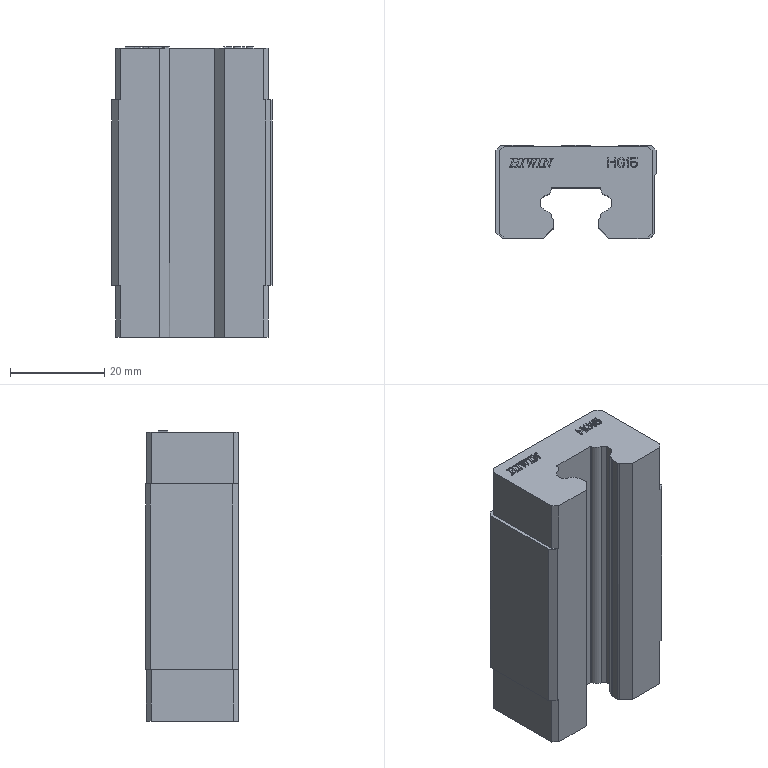Part | NX | features BREP 1 | 1 solid | 424 faces | box 34 x 19.7 x 61.7 mm | volume 31747 mm3 | plane 297 | cylinder 76 | spline 51 | commonest cylinder face diameters 0.8 x8 4 x8 3.24 x4 0.062 x3 0.05 x2 0.095 x2